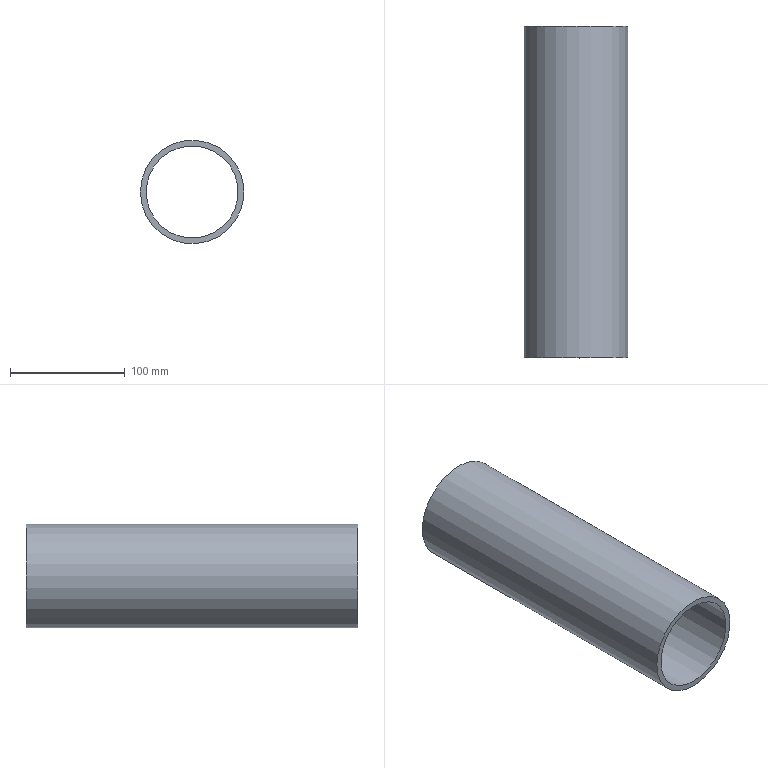Part | STEP file | SN10_002_009-02_TUBO | 1 solid | 4 faces | box 90 x 288.6 x 90 mm | volume 385332 mm3 | cylinder 2 | plane 2 | commonest cylinder face diameters 80 x1 90 x1
STEP:
#1=CARTESIAN_POINT('',(0.,0.,0.));
#2=DIRECTION('',(0.,0.,1.));
#3=DIRECTION('',(1.,0.,0.));
#4=AXIS2_PLACEMENT_3D('',#1,#2,#3);
#5=CARTESIAN_POINT('',(955.,-15.7,0.));
#6=VERTEX_POINT('',#5);
#7=CARTESIAN_POINT('',(1000.,-15.7,0.));
#8=DIRECTION('',(0.,1.,0.));
#9=DIRECTION('',(1.,0.,0.));
#10=AXIS2_PLACEMENT_3D('',#7,#8,#9);
#11=CIRCLE('',#10,45.);
#12=CARTESIAN_POINT('',(1000.,-160.,0.));
#13=DIRECTION('',(0.,1.,0.));
#14=DIRECTION('',(1.,0.,0.));
#15=AXIS2_PLACEMENT_3D('',#12,#13,#14);
#16=CYLINDRICAL_SURFACE('',#15,45.);
#17=CARTESIAN_POINT('',(0.,144.3));
#18=DIRECTION('',(1.,0.));
#19=VECTOR('',#18,1.);
#20=LINE('',#17,#19);
#21=(GEOMETRIC_REPRESENTATION_CONTEXT(2)PARAMETRIC_REPRESENTATION_CONTEXT()REPRESENTATION_CONTEXT('',''));
#22=DEFINITIONAL_REPRESENTATION('',(#20),#21);
#23=PCURVE('',#16,#22);
#24=CARTESIAN_POINT('',(0.,-15.7,0.));
#25=DIRECTION('',(0.,1.,0.));
#26=DIRECTION('',(0.,0.,1.));
#27=AXIS2_PLACEMENT_3D('',#24,#25,#26);
#28=PLANE('',#27);
#29=CARTESIAN_POINT('',(0.,1000.));
#30=DIRECTION('',(0.,1.));
#31=AXIS2_PLACEMENT_2D('',#29,#30);
#32=CIRCLE('',#31,45.);
#33=(GEOMETRIC_REPRESENTATION_CONTEXT(2)PARAMETRIC_REPRESENTATION_CONTEXT()REPRESENTATION_CONTEXT('',''));
#34=DEFINITIONAL_REPRESENTATION('',(#32),#33);
#35=PCURVE('',#28,#34);
#36=SURFACE_CURVE('',#11,(#23,#35),.PCURVE_S1.);
#37=EDGE_CURVE('',#6,#6,#36,.T.);
#38=ORIENTED_EDGE('',*,*,#37,.F.);
#39=CARTESIAN_POINT('',(955.,-304.3,0.));
#40=VERTEX_POINT('',#39);
#41=CARTESIAN_POINT('',(955.,-304.3,0.));
#42=CARTESIAN_POINT('',(955.,-15.7,0.));
#43=B_SPLINE_CURVE_WITH_KNOTS('',1,(#41,#42),.UNSPECIFIED.,.F.,.F.,(2,2),(-144.3,144.3),.PIECEWISE_BEZIER_KNOTS.);
#44=CARTESIAN_POINT('',(3.142,0.));
#45=DIRECTION('',(0.,1.));
#46=VECTOR('',#45,1.);
#47=LINE('',#44,#46);
#48=(GEOMETRIC_REPRESENTATION_CONTEXT(2)PARAMETRIC_REPRESENTATION_CONTEXT()REPRESENTATION_CONTEXT('',''));
#49=DEFINITIONAL_REPRESENTATION('',(#47),#48);
#50=PCURVE('',#16,#49);
#51=CARTESIAN_POINT('',(9.425,0.));
#52=DIRECTION('',(0.,1.));
#53=VECTOR('',#52,1.);
#54=LINE('',#51,#53);
#55=(GEOMETRIC_REPRESENTATION_CONTEXT(2)PARAMETRIC_REPRESENTATION_CONTEXT()REPRESENTATION_CONTEXT('',''));
#56=DEFINITIONAL_REPRESENTATION('',(#54),#55);
#57=PCURVE('',#16,#56);
#58=SEAM_CURVE('',#43,(#50,#57),.PCURVE_S1.);
#59=EDGE_CURVE('',#40,#6,#58,.T.);
#60=ORIENTED_EDGE('',*,*,#59,.F.);
#61=CARTESIAN_POINT('',(1000.,-304.3,0.));
#62=DIRECTION('',(0.,1.,0.));
#63=DIRECTION('',(1.,0.,0.));
#64=AXIS2_PLACEMENT_3D('',#61,#62,#63);
#65=CIRCLE('',#64,45.);
#66=CARTESIAN_POINT('',(0.,-144.3));
#67=DIRECTION('',(1.,0.));
#68=VECTOR('',#67,1.);
#69=LINE('',#66,#68);
#70=(GEOMETRIC_REPRESENTATION_CONTEXT(2)PARAMETRIC_REPRESENTATION_CONTEXT()REPRESENTATION_CONTEXT('',''));
#71=DEFINITIONAL_REPRESENTATION('',(#69),#70);
#72=PCURVE('',#16,#71);
#73=CARTESIAN_POINT('',(0.,-304.3,0.));
#74=DIRECTION('',(0.,1.,0.));
#75=DIRECTION('',(0.,0.,1.));
#76=AXIS2_PLACEMENT_3D('',#73,#74,#75);
#77=PLANE('',#76);
#78=CARTESIAN_POINT('',(0.,1000.));
#79=DIRECTION('',(0.,1.));
#80=AXIS2_PLACEMENT_2D('',#78,#79);
#81=CIRCLE('',#80,45.);
#82=(GEOMETRIC_REPRESENTATION_CONTEXT(2)PARAMETRIC_REPRESENTATION_CONTEXT()REPRESENTATION_CONTEXT('',''));
#83=DEFINITIONAL_REPRESENTATION('',(#81),#82);
#84=PCURVE('',#77,#83);
#85=SURFACE_CURVE('',#65,(#72,#84),.PCURVE_S1.);
#86=EDGE_CURVE('',#40,#40,#85,.T.);
#87=ORIENTED_EDGE('',*,*,#86,.T.);
#88=ORIENTED_EDGE('',*,*,#59,.T.);
#89=EDGE_LOOP('',(#38,#60,#87,#88));
#90=FACE_BOUND('',#89,.T.);
#91=ADVANCED_FACE('',(#90),#16,.T.);
#92=CARTESIAN_POINT('',(1000.,-15.7,-40.));
#93=VERTEX_POINT('',#92);
#94=CARTESIAN_POINT('',(1000.,-15.7,0.));
#95=DIRECTION('',(0.,1.,0.));
#96=DIRECTION('',(1.,0.,0.));
#97=AXIS2_PLACEMENT_3D('',#94,#95,#96);
#98=CIRCLE('',#97,40.);
#99=CARTESIAN_POINT('',(1000.,-160.,0.));
#100=DIRECTION('',(0.,1.,0.));
#101=DIRECTION('',(0.,0.,1.));
#102=AXIS2_PLACEMENT_3D('',#99,#100,#101);
#103=CYLINDRICAL_SURFACE('',#102,40.);
#104=CARTESIAN_POINT('',(1.571,144.3));
#105=DIRECTION('',(1.,0.));
#106=VECTOR('',#105,1.);
#107=LINE('',#104,#106);
#108=(GEOMETRIC_REPRESENTATION_CONTEXT(2)PARAMETRIC_REPRESENTATION_CONTEXT()REPRESENTATION_CONTEXT('',''));
#109=DEFINITIONAL_REPRESENTATION('',(#107),#108);
#110=PCURVE('',#103,#109);
#111=CARTESIAN_POINT('',(0.,1000.));
#112=DIRECTION('',(0.,1.));
#113=AXIS2_PLACEMENT_2D('',#111,#112);
#114=CIRCLE('',#113,40.);
#115=(GEOMETRIC_REPRESENTATION_CONTEXT(2)PARAMETRIC_REPRESENTATION_CONTEXT()REPRESENTATION_CONTEXT('',''));
#116=DEFINITIONAL_REPRESENTATION('',(#114),#115);
#117=PCURVE('',#28,#116);
#118=SURFACE_CURVE('',#98,(#110,#117),.PCURVE_S1.);
#119=EDGE_CURVE('',#93,#93,#118,.T.);
#120=ORIENTED_EDGE('',*,*,#119,.F.);
#121=CARTESIAN_POINT('',(1000.,-304.3,-40.));
#122=VERTEX_POINT('',#121);
#123=CARTESIAN_POINT('',(1000.,-304.3,-40.));
#124=CARTESIAN_POINT('',(1000.,-15.7,-40.));
#125=B_SPLINE_CURVE_WITH_KNOTS('',1,(#123,#124),.UNSPECIFIED.,.F.,.F.,(2,2),(-144.3,144.3),.PIECEWISE_BEZIER_KNOTS.);
#126=CARTESIAN_POINT('',(3.142,0.));
#127=DIRECTION('',(0.,1.));
#128=VECTOR('',#127,1.);
#129=LINE('',#126,#128);
#130=(GEOMETRIC_REPRESENTATION_CONTEXT(2)PARAMETRIC_REPRESENTATION_CONTEXT()REPRESENTATION_CONTEXT('',''));
#131=DEFINITIONAL_REPRESENTATION('',(#129),#130);
#132=PCURVE('',#103,#131);
#133=CARTESIAN_POINT('',(9.425,0.));
#134=DIRECTION('',(0.,1.));
#135=VECTOR('',#134,1.);
#136=LINE('',#133,#135);
#137=(GEOMETRIC_REPRESENTATION_CONTEXT(2)PARAMETRIC_REPRESENTATION_CONTEXT()REPRESENTATION_CONTEXT('',''));
#138=DEFINITIONAL_REPRESENTATION('',(#136),#137);
#139=PCURVE('',#103,#138);
#140=SEAM_CURVE('',#125,(#132,#139),.PCURVE_S1.);
#141=EDGE_CURVE('',#122,#93,#140,.T.);
#142=ORIENTED_EDGE('',*,*,#141,.F.);
#143=CARTESIAN_POINT('',(1000.,-304.3,0.));
#144=DIRECTION('',(0.,1.,0.));
#145=DIRECTION('',(1.,0.,0.));
#146=AXIS2_PLACEMENT_3D('',#143,#144,#145);
#147=CIRCLE('',#146,40.);
#148=CARTESIAN_POINT('',(1.571,-144.3));
#149=DIRECTION('',(1.,0.));
#150=VECTOR('',#149,1.);
#151=LINE('',#148,#150);
#152=(GEOMETRIC_REPRESENTATION_CONTEXT(2)PARAMETRIC_REPRESENTATION_CONTEXT()REPRESENTATION_CONTEXT('',''));
#153=DEFINITIONAL_REPRESENTATION('',(#151),#152);
#154=PCURVE('',#103,#153);
#155=CARTESIAN_POINT('',(0.,1000.));
#156=DIRECTION('',(0.,1.));
#157=AXIS2_PLACEMENT_2D('',#155,#156);
#158=CIRCLE('',#157,40.);
#159=(GEOMETRIC_REPRESENTATION_CONTEXT(2)PARAMETRIC_REPRESENTATION_CONTEXT()REPRESENTATION_CONTEXT('',''));
#160=DEFINITIONAL_REPRESENTATION('',(#158),#159);
#161=PCURVE('',#77,#160);
#162=SURFACE_CURVE('',#147,(#154,#161),.PCURVE_S1.);
#163=EDGE_CURVE('',#122,#122,#162,.T.);
#164=ORIENTED_EDGE('',*,*,#163,.T.);
#165=ORIENTED_EDGE('',*,*,#141,.T.);
#166=EDGE_LOOP('',(#120,#142,#164,#165));
#167=FACE_BOUND('',#166,.F.);
#168=ADVANCED_FACE('',(#167),#103,.F.);
#169=ORIENTED_EDGE('',*,*,#86,.F.);
#170=EDGE_LOOP('',(#169));
#171=FACE_BOUND('',#170,.T.);
#172=ORIENTED_EDGE('',*,*,#163,.T.);
#173=EDGE_LOOP('',(#172));
#174=FACE_BOUND('',#173,.T.);
#175=ADVANCED_FACE('',(#171,#174),#77,.F.);
#176=ORIENTED_EDGE('',*,*,#37,.T.);
#177=EDGE_LOOP('',(#176));
#178=FACE_BOUND('',#177,.T.);
#179=ORIENTED_EDGE('',*,*,#119,.F.);
#180=EDGE_LOOP('',(#179));
#181=FACE_BOUND('',#180,.T.);
#182=ADVANCED_FACE('',(#178,#181),#28,.T.);
#183=CLOSED_SHELL('',(#91,#168,#175,#182));
#184=MANIFOLD_SOLID_BREP('',#183);
#185=(LENGTH_UNIT()NAMED_UNIT(*)SI_UNIT(.MILLI.,.METRE.));
#186=UNCERTAINTY_MEASURE_WITH_UNIT(LENGTH_MEASURE(0.00001),#185,'','');
#187=(NAMED_UNIT(*)PLANE_ANGLE_UNIT()SI_UNIT($,.RADIAN.));
#188=(NAMED_UNIT(*)SI_UNIT($,.STERADIAN.)SOLID_ANGLE_UNIT());
#189=(GEOMETRIC_REPRESENTATION_CONTEXT(3)GLOBAL_UNCERTAINTY_ASSIGNED_CONTEXT((#186))GLOBAL_UNIT_ASSIGNED_CONTEXT((#185,#187,#188))REPRESENTATION_CONTEXT('',''));
#190=ADVANCED_BREP_SHAPE_REPRESENTATION('',(#4,#184),#189);